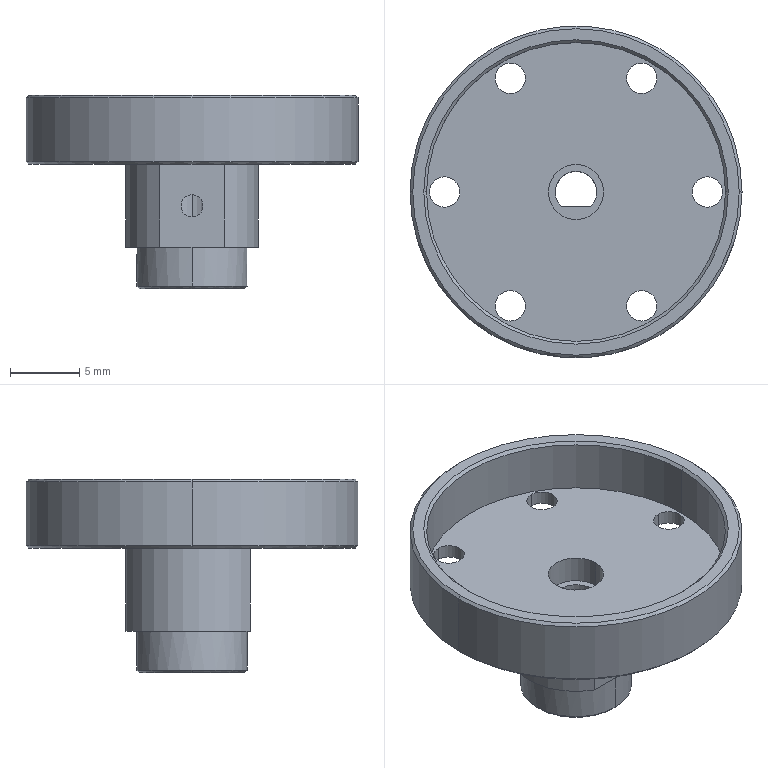Part | 1 solid | 49 faces | box 24 x 24 x 14 mm | volume 1249 mm3 | cylinder 29 | cone 12 | plane 8 | commonest cylinder face diameters 2.2 x12 1.25 x4 1.6 x2 3 x2 4 x2 8 x2
STEP:
#1=CARTESIAN_POINT('',(-11.8,0.,-5.));
#2=VERTEX_POINT('',#1);
#3=CARTESIAN_POINT('',(11.8,0.,-5.));
#4=VERTEX_POINT('',#3);
#5=CARTESIAN_POINT('',(0.,0.,-5.));
#6=DIRECTION('',(0.,0.,-1.));
#7=DIRECTION('',(0.,1.,0.));
#8=AXIS2_PLACEMENT_3D('',#5,#6,#7);
#9=CIRCLE('',#8,11.8);
#10=EDGE_CURVE('',#2,#4,#9,.T.);
#11=ORIENTED_EDGE('',*,*,#10,.F.);
#12=CARTESIAN_POINT('',(-12.,0.,-4.8));
#13=VERTEX_POINT('',#12);
#14=CARTESIAN_POINT('',(-12.,0.,-4.8));
#15=DIRECTION('',(-0.7071,0.,0.7071));
#16=VECTOR('',#15,1000.);
#17=LINE('',#14,#16);
#18=EDGE_CURVE('',#2,#13,#17,.T.);
#19=ORIENTED_EDGE('',*,*,#18,.T.);
#20=CARTESIAN_POINT('',(12.,0.,-4.8));
#21=VERTEX_POINT('',#20);
#22=CARTESIAN_POINT('',(0.,0.,-4.8));
#23=DIRECTION('',(0.,0.,1.));
#24=DIRECTION('',(-1.,0.,0.));
#25=AXIS2_PLACEMENT_3D('',#22,#23,#24);
#26=CIRCLE('',#25,12.);
#27=EDGE_CURVE('',#21,#13,#26,.T.);
#28=ORIENTED_EDGE('',*,*,#27,.F.);
#29=CARTESIAN_POINT('',(12.,0.,-4.8));
#30=DIRECTION('',(0.7071,0.,0.7071));
#31=VECTOR('',#30,1000.);
#32=LINE('',#29,#31);
#33=EDGE_CURVE('',#4,#21,#32,.T.);
#34=ORIENTED_EDGE('',*,*,#33,.F.);
#35=EDGE_LOOP('',(#11,#19,#28,#34));
#36=FACE_BOUND('',#35,.T.);
#37=CARTESIAN_POINT('',(0.,0.,-4.8));
#38=DIRECTION('',(0.,0.,1.));
#39=DIRECTION('',(-1.,0.,0.));
#40=AXIS2_PLACEMENT_3D('',#37,#38,#39);
#41=CONICAL_SURFACE('',#40,12.,0.7854);
#42=ADVANCED_FACE('',(#36),#41,.T.);
#43=CARTESIAN_POINT('',(-10.8,0.,-0.2));
#44=VERTEX_POINT('',#43);
#45=CARTESIAN_POINT('',(10.8,0.,-0.2));
#46=VERTEX_POINT('',#45);
#47=CARTESIAN_POINT('',(0.,0.,-0.2));
#48=DIRECTION('',(0.,0.,1.));
#49=DIRECTION('',(1.,0.,0.));
#50=AXIS2_PLACEMENT_3D('',#47,#48,#49);
#51=CIRCLE('',#50,10.8);
#52=EDGE_CURVE('',#44,#46,#51,.T.);
#53=ORIENTED_EDGE('',*,*,#52,.F.);
#54=CARTESIAN_POINT('',(-11.,0.,0.));
#55=VERTEX_POINT('',#54);
#56=CARTESIAN_POINT('',(-10.8,0.,-0.2));
#57=DIRECTION('',(-0.7071,0.,0.7071));
#58=VECTOR('',#57,1000.);
#59=LINE('',#56,#58);
#60=EDGE_CURVE('',#44,#55,#59,.T.);
#61=ORIENTED_EDGE('',*,*,#60,.T.);
#62=CARTESIAN_POINT('',(11.,0.,0.));
#63=VERTEX_POINT('',#62);
#64=CARTESIAN_POINT('',(0.,0.,0.));
#65=DIRECTION('',(0.,0.,-1.));
#66=DIRECTION('',(1.,0.,0.));
#67=AXIS2_PLACEMENT_3D('',#64,#65,#66);
#68=CIRCLE('',#67,11.);
#69=EDGE_CURVE('',#63,#55,#68,.T.);
#70=ORIENTED_EDGE('',*,*,#69,.F.);
#71=CARTESIAN_POINT('',(10.8,0.,-0.2));
#72=DIRECTION('',(0.7071,0.,0.7071));
#73=VECTOR('',#72,1000.);
#74=LINE('',#71,#73);
#75=EDGE_CURVE('',#46,#63,#74,.T.);
#76=ORIENTED_EDGE('',*,*,#75,.F.);
#77=EDGE_LOOP('',(#53,#61,#70,#76));
#78=FACE_BOUND('',#77,.T.);
#79=CARTESIAN_POINT('',(0.,0.,-0.2));
#80=DIRECTION('',(0.,0.,1.));
#81=DIRECTION('',(-1.,0.,0.));
#82=AXIS2_PLACEMENT_3D('',#79,#80,#81);
#83=CONICAL_SURFACE('',#82,10.8,0.7854);
#84=ADVANCED_FACE('',(#78),#83,.F.);
#85=CARTESIAN_POINT('',(11.8,0.,0.));
#86=VERTEX_POINT('',#85);
#87=CARTESIAN_POINT('',(-11.8,0.,0.));
#88=VERTEX_POINT('',#87);
#89=CARTESIAN_POINT('',(0.,0.,0.));
#90=DIRECTION('',(0.,0.,1.));
#91=DIRECTION('',(1.,0.,0.));
#92=AXIS2_PLACEMENT_3D('',#89,#90,#91);
#93=CIRCLE('',#92,11.8);
#94=EDGE_CURVE('',#86,#88,#93,.T.);
#95=ORIENTED_EDGE('',*,*,#94,.F.);
#96=CARTESIAN_POINT('',(12.,0.,-0.2));
#97=VERTEX_POINT('',#96);
#98=CARTESIAN_POINT('',(11.8,0.,0.));
#99=DIRECTION('',(0.7071,0.,-0.7071));
#100=VECTOR('',#99,1000.);
#101=LINE('',#98,#100);
#102=EDGE_CURVE('',#86,#97,#101,.T.);
#103=ORIENTED_EDGE('',*,*,#102,.T.);
#104=CARTESIAN_POINT('',(-12.,0.,-0.2));
#105=VERTEX_POINT('',#104);
#106=CARTESIAN_POINT('',(0.,0.,-0.2));
#107=DIRECTION('',(0.,0.,-1.));
#108=DIRECTION('',(1.,0.,0.));
#109=AXIS2_PLACEMENT_3D('',#106,#107,#108);
#110=CIRCLE('',#109,12.);
#111=EDGE_CURVE('',#105,#97,#110,.T.);
#112=ORIENTED_EDGE('',*,*,#111,.F.);
#113=CARTESIAN_POINT('',(-11.8,0.,0.));
#114=DIRECTION('',(-0.7071,0.,-0.7071));
#115=VECTOR('',#114,1000.);
#116=LINE('',#113,#115);
#117=EDGE_CURVE('',#88,#105,#116,.T.);
#118=ORIENTED_EDGE('',*,*,#117,.F.);
#119=EDGE_LOOP('',(#95,#103,#112,#118));
#120=FACE_BOUND('',#119,.T.);
#121=CARTESIAN_POINT('',(0.,0.,0.));
#122=DIRECTION('',(0.,0.,-1.));
#123=DIRECTION('',(1.,0.,0.));
#124=AXIS2_PLACEMENT_3D('',#121,#122,#123);
#125=CONICAL_SURFACE('',#124,11.8,0.7854);
#126=ADVANCED_FACE('',(#120),#125,.T.);
#127=CARTESIAN_POINT('',(-3.8,0.,-14.));
#128=VERTEX_POINT('',#127);
#129=CARTESIAN_POINT('',(3.8,0.,-14.));
#130=VERTEX_POINT('',#129);
#131=CARTESIAN_POINT('',(0.,0.,-14.));
#132=DIRECTION('',(0.,0.,-1.));
#133=DIRECTION('',(0.,1.,0.));
#134=AXIS2_PLACEMENT_3D('',#131,#132,#133);
#135=CIRCLE('',#134,3.8);
#136=EDGE_CURVE('',#128,#130,#135,.T.);
#137=ORIENTED_EDGE('',*,*,#136,.F.);
#138=CARTESIAN_POINT('',(-4.,0.,-13.8));
#139=VERTEX_POINT('',#138);
#140=CARTESIAN_POINT('',(-3.8,0.,-14.));
#141=DIRECTION('',(-0.7071,0.,0.7071));
#142=VECTOR('',#141,1000.);
#143=LINE('',#140,#142);
#144=EDGE_CURVE('',#128,#139,#143,.T.);
#145=ORIENTED_EDGE('',*,*,#144,.T.);
#146=CARTESIAN_POINT('',(0.,4.,-13.8));
#147=VERTEX_POINT('',#146);
#148=CARTESIAN_POINT('',(0.,0.,-13.8));
#149=DIRECTION('',(0.,0.,1.));
#150=DIRECTION('',(-1.,0.,0.));
#151=AXIS2_PLACEMENT_3D('',#148,#149,#150);
#152=CIRCLE('',#151,4.);
#153=EDGE_CURVE('',#147,#139,#152,.T.);
#154=ORIENTED_EDGE('',*,*,#153,.F.);
#155=CARTESIAN_POINT('',(4.,0.,-13.8));
#156=VERTEX_POINT('',#155);
#157=CARTESIAN_POINT('',(0.,0.,-13.8));
#158=DIRECTION('',(0.,0.,1.));
#159=DIRECTION('',(-1.,0.,0.));
#160=AXIS2_PLACEMENT_3D('',#157,#158,#159);
#161=CIRCLE('',#160,4.);
#162=EDGE_CURVE('',#156,#147,#161,.T.);
#163=ORIENTED_EDGE('',*,*,#162,.F.);
#164=CARTESIAN_POINT('',(3.8,0.,-14.));
#165=DIRECTION('',(0.7071,0.,0.7071));
#166=VECTOR('',#165,1000.);
#167=LINE('',#164,#166);
#168=EDGE_CURVE('',#130,#156,#167,.T.);
#169=ORIENTED_EDGE('',*,*,#168,.F.);
#170=EDGE_LOOP('',(#137,#145,#154,#163,#169));
#171=FACE_BOUND('',#170,.T.);
#172=CARTESIAN_POINT('',(0.,0.,-14.));
#173=DIRECTION('',(0.,0.,1.));
#174=DIRECTION('',(-1.,0.,0.));
#175=AXIS2_PLACEMENT_3D('',#172,#173,#174);
#176=CONICAL_SURFACE('',#175,3.8,0.7854);
#177=ADVANCED_FACE('',(#171),#176,.T.);
#178=CARTESIAN_POINT('',(-2.,0.,-6.));
#179=VERTEX_POINT('',#178);
#180=CARTESIAN_POINT('',(2.,0.,-6.));
#181=VERTEX_POINT('',#180);
#182=CARTESIAN_POINT('',(0.,0.,-6.));
#183=DIRECTION('',(0.,0.,1.));
#184=DIRECTION('',(1.,0.,0.));
#185=AXIS2_PLACEMENT_3D('',#182,#183,#184);
#186=CIRCLE('',#185,2.);
#187=EDGE_CURVE('',#179,#181,#186,.T.);
#188=ORIENTED_EDGE('',*,*,#187,.F.);
#189=CARTESIAN_POINT('',(-2.,0.,-4.));
#190=VERTEX_POINT('',#189);
#191=CARTESIAN_POINT('',(-2.,0.,-6.));
#192=DIRECTION('',(0.,0.,1.));
#193=VECTOR('',#192,1000.);
#194=LINE('',#191,#193);
#195=EDGE_CURVE('',#179,#190,#194,.T.);
#196=ORIENTED_EDGE('',*,*,#195,.T.);
#197=CARTESIAN_POINT('',(2.,0.,-4.));
#198=VERTEX_POINT('',#197);
#199=CARTESIAN_POINT('',(0.,0.,-4.));
#200=DIRECTION('',(0.,0.,1.));
#201=DIRECTION('',(1.,0.,0.));
#202=AXIS2_PLACEMENT_3D('',#199,#200,#201);
#203=CIRCLE('',#202,2.);
#204=EDGE_CURVE('',#190,#198,#203,.T.);
#205=ORIENTED_EDGE('',*,*,#204,.T.);
#206=CARTESIAN_POINT('',(2.,0.,-6.));
#207=DIRECTION('',(0.,0.,1.));
#208=VECTOR('',#207,1000.);
#209=LINE('',#206,#208);
#210=EDGE_CURVE('',#181,#198,#209,.T.);
#211=ORIENTED_EDGE('',*,*,#210,.F.);
#212=EDGE_LOOP('',(#188,#196,#205,#211));
#213=FACE_BOUND('',#212,.T.);
#214=CARTESIAN_POINT('',(0.,0.,-6.));
#215=DIRECTION('',(0.,0.,1.));
#216=DIRECTION('',(-1.,0.,0.));
#217=AXIS2_PLACEMENT_3D('',#214,#215,#216);
#218=CYLINDRICAL_SURFACE('',#217,2.);
#219=ADVANCED_FACE('',(#213),#218,.F.);
#220=ORIENTED_EDGE('',*,*,#111,.T.);
#221=CARTESIAN_POINT('',(12.,0.,0.));
#222=DIRECTION('',(0.,0.,-1.));
#223=VECTOR('',#222,1000.);
#224=LINE('',#221,#223);
#225=EDGE_CURVE('',#97,#21,#224,.T.);
#226=ORIENTED_EDGE('',*,*,#225,.T.);
#227=ORIENTED_EDGE('',*,*,#27,.T.);
#228=CARTESIAN_POINT('',(-12.,0.,0.));
#229=DIRECTION('',(0.,0.,-1.));
#230=VECTOR('',#229,1000.);
#231=LINE('',#228,#230);
#232=EDGE_CURVE('',#105,#13,#231,.T.);
#233=ORIENTED_EDGE('',*,*,#232,.F.);
#234=EDGE_LOOP('',(#220,#226,#227,#233));
#235=FACE_BOUND('',#234,.T.);
#236=CARTESIAN_POINT('',(0.,0.,0.));
#237=DIRECTION('',(0.,0.,-1.));
#238=DIRECTION('',(1.,0.,0.));
#239=AXIS2_PLACEMENT_3D('',#236,#237,#238);
#240=CYLINDRICAL_SURFACE('',#239,12.);
#241=ADVANCED_FACE('',(#235),#240,.T.);
#242=ORIENTED_EDGE('',*,*,#52,.T.);
#243=CARTESIAN_POINT('',(10.8,0.,-4.));
#244=VERTEX_POINT('',#243);
#245=CARTESIAN_POINT('',(10.8,0.,0.));
#246=DIRECTION('',(0.,0.,-1.));
#247=VECTOR('',#246,1000.);
#248=LINE('',#245,#247);
#249=EDGE_CURVE('',#46,#244,#248,.T.);
#250=ORIENTED_EDGE('',*,*,#249,.T.);
#251=CARTESIAN_POINT('',(-10.8,0.,-4.));
#252=VERTEX_POINT('',#251);
#253=CARTESIAN_POINT('',(0.,0.,-4.));
#254=DIRECTION('',(0.,0.,-1.));
#255=DIRECTION('',(0.,1.,0.));
#256=AXIS2_PLACEMENT_3D('',#253,#254,#255);
#257=CIRCLE('',#256,10.8);
#258=EDGE_CURVE('',#244,#252,#257,.T.);
#259=ORIENTED_EDGE('',*,*,#258,.T.);
#260=CARTESIAN_POINT('',(-10.8,0.,0.));
#261=DIRECTION('',(0.,0.,-1.));
#262=VECTOR('',#261,1000.);
#263=LINE('',#260,#262);
#264=EDGE_CURVE('',#44,#252,#263,.T.);
#265=ORIENTED_EDGE('',*,*,#264,.F.);
#266=EDGE_LOOP('',(#242,#250,#259,#265));
#267=FACE_BOUND('',#266,.T.);
#268=CARTESIAN_POINT('',(0.,0.,0.));
#269=DIRECTION('',(0.,0.,-1.));
#270=DIRECTION('',(1.,0.,0.));
#271=AXIS2_PLACEMENT_3D('',#268,#269,#270);
#272=CYLINDRICAL_SURFACE('',#271,10.8);
#273=ADVANCED_FACE('',(#267),#272,.F.);
#274=CARTESIAN_POINT('',(-2.75,-0.625,-9.75));
#275=VERTEX_POINT('',#274);
#276=CARTESIAN_POINT('',(-2.75,0.625,-9.75));
#277=VERTEX_POINT('',#276);
#278=CARTESIAN_POINT('',(-2.75,0.,-9.75));
#279=DIRECTION('',(0.,0.,-1.));
#280=DIRECTION('',(0.,1.,0.));
#281=AXIS2_PLACEMENT_3D('',#278,#279,#280);
#282=CIRCLE('',#281,0.625);
#283=EDGE_CURVE('',#275,#277,#282,.T.);
#284=ORIENTED_EDGE('',*,*,#283,.F.);
#285=CARTESIAN_POINT('',(-2.75,-0.625,-14.));
#286=VERTEX_POINT('',#285);
#287=CARTESIAN_POINT('',(-2.75,-0.625,-14.));
#288=DIRECTION('',(0.,0.,-1.));
#289=VECTOR('',#288,1000.);
#290=LINE('',#287,#289);
#291=EDGE_CURVE('',#275,#286,#290,.T.);
#292=ORIENTED_EDGE('',*,*,#291,.T.);
#293=CARTESIAN_POINT('',(-2.75,0.625,-14.));
#294=VERTEX_POINT('',#293);
#295=CARTESIAN_POINT('',(-2.75,0.,-14.));
#296=DIRECTION('',(0.,0.,-1.));
#297=DIRECTION('',(0.,1.,0.));
#298=AXIS2_PLACEMENT_3D('',#295,#296,#297);
#299=CIRCLE('',#298,0.625);
#300=EDGE_CURVE('',#286,#294,#299,.T.);
#301=ORIENTED_EDGE('',*,*,#300,.T.);
#302=CARTESIAN_POINT('',(-2.75,0.625,-14.));
#303=DIRECTION('',(0.,0.,-1.));
#304=VECTOR('',#303,1000.);
#305=LINE('',#302,#304);
#306=EDGE_CURVE('',#277,#294,#305,.T.);
#307=ORIENTED_EDGE('',*,*,#306,.F.);
#308=EDGE_LOOP('',(#284,#292,#301,#307));
#309=FACE_BOUND('',#308,.T.);
#310=CARTESIAN_POINT('',(-2.75,0.,-14.));
#311=DIRECTION('',(0.,0.,-1.));
#312=DIRECTION('',(0.,-1.,0.));
#313=AXIS2_PLACEMENT_3D('',#310,#311,#312);
#314=CYLINDRICAL_SURFACE('',#313,0.625);
#315=ADVANCED_FACE('',(#309),#314,.F.);
#316=CARTESIAN_POINT('',(-2.75,0.,-9.374));
#317=VERTEX_POINT('',#316);
#318=CARTESIAN_POINT('',(-2.75,0.625,-9.75));
#319=DIRECTION('',(0.,0.8572,-0.515));
#320=VECTOR('',#319,1000.);
#321=LINE('',#318,#320);
#322=EDGE_CURVE('',#317,#277,#321,.T.);
#323=ORIENTED_EDGE('',*,*,#322,.F.);
#324=CARTESIAN_POINT('',(-2.75,-0.625,-9.75));
#325=DIRECTION('',(0.,-0.8572,-0.515));
#326=VECTOR('',#325,1000.);
#327=LINE('',#324,#326);
#328=EDGE_CURVE('',#317,#275,#327,.T.);
#329=ORIENTED_EDGE('',*,*,#328,.T.);
#330=ORIENTED_EDGE('',*,*,#283,.T.);
#331=EDGE_LOOP('',(#323,#329,#330));
#332=FACE_BOUND('',#331,.T.);
#333=CARTESIAN_POINT('',(-2.75,0.,-9.75));
#334=DIRECTION('',(0.,0.,-1.));
#335=DIRECTION('',(0.,-1.,0.));
#336=AXIS2_PLACEMENT_3D('',#333,#334,#335);
#337=CONICAL_SURFACE('',#336,0.625,1.03);
#338=ADVANCED_FACE('',(#332),#337,.F.);
#339=CARTESIAN_POINT('',(2.75,-0.625,-9.75));
#340=VERTEX_POINT('',#339);
#341=CARTESIAN_POINT('',(2.75,0.625,-9.75));
#342=VERTEX_POINT('',#341);
#343=CARTESIAN_POINT('',(2.75,0.,-9.75));
#344=DIRECTION('',(0.,0.,-1.));
#345=DIRECTION('',(0.,1.,0.));
#346=AXIS2_PLACEMENT_3D('',#343,#344,#345);
#347=CIRCLE('',#346,0.625);
#348=EDGE_CURVE('',#340,#342,#347,.T.);
#349=ORIENTED_EDGE('',*,*,#348,.F.);
#350=CARTESIAN_POINT('',(2.75,-0.625,-14.));
#351=VERTEX_POINT('',#350);
#352=CARTESIAN_POINT('',(2.75,-0.625,-14.));
#353=DIRECTION('',(0.,0.,-1.));
#354=VECTOR('',#353,1000.);
#355=LINE('',#352,#354);
#356=EDGE_CURVE('',#340,#351,#355,.T.);
#357=ORIENTED_EDGE('',*,*,#356,.T.);
#358=CARTESIAN_POINT('',(2.75,0.625,-14.));
#359=VERTEX_POINT('',#358);
#360=CARTESIAN_POINT('',(2.75,0.,-14.));
#361=DIRECTION('',(0.,0.,-1.));
#362=DIRECTION('',(0.,1.,0.));
#363=AXIS2_PLACEMENT_3D('',#360,#361,#362);
#364=CIRCLE('',#363,0.625);
#365=EDGE_CURVE('',#351,#359,#364,.T.);
#366=ORIENTED_EDGE('',*,*,#365,.T.);
#367=CARTESIAN_POINT('',(2.75,0.625,-14.));
#368=DIRECTION('',(0.,0.,-1.));
#369=VECTOR('',#368,1000.);
#370=LINE('',#367,#369);
#371=EDGE_CURVE('',#342,#359,#370,.T.);
#372=ORIENTED_EDGE('',*,*,#371,.F.);
#373=EDGE_LOOP('',(#349,#357,#366,#372));
#374=FACE_BOUND('',#373,.T.);
#375=CARTESIAN_POINT('',(2.75,0.,-14.));
#376=DIRECTION('',(0.,0.,-1.));
#377=DIRECTION('',(0.,-1.,0.));
#378=AXIS2_PLACEMENT_3D('',#375,#376,#377);
#379=CYLINDRICAL_SURFACE('',#378,0.625);
#380=ADVANCED_FACE('',(#374),#379,.F.);
#381=CARTESIAN_POINT('',(2.75,0.,-9.374));
#382=VERTEX_POINT('',#381);
#383=CARTESIAN_POINT('',(2.75,0.625,-9.75));
#384=DIRECTION('',(0.,0.8572,-0.515));
#385=VECTOR('',#384,1000.);
#386=LINE('',#383,#385);
#387=EDGE_CURVE('',#382,#342,#386,.T.);
#388=ORIENTED_EDGE('',*,*,#387,.F.);
#389=CARTESIAN_POINT('',(2.75,-0.625,-9.75));
#390=DIRECTION('',(0.,-0.8572,-0.515));
#391=VECTOR('',#390,1000.);
#392=LINE('',#389,#391);
#393=EDGE_CURVE('',#382,#340,#392,.T.);
#394=ORIENTED_EDGE('',*,*,#393,.T.);
#395=ORIENTED_EDGE('',*,*,#348,.T.);
#396=EDGE_LOOP('',(#388,#394,#395));
#397=FACE_BOUND('',#396,.T.);
#398=CARTESIAN_POINT('',(2.75,0.,-9.75));
#399=DIRECTION('',(0.,0.,-1.));
#400=DIRECTION('',(0.,-1.,0.));
#401=AXIS2_PLACEMENT_3D('',#398,#399,#400);
#402=CONICAL_SURFACE('',#401,0.625,1.03);
#403=ADVANCED_FACE('',(#397),#402,.F.);
#404=CARTESIAN_POINT('',(0.,-1.05,-7.2));
#405=VERTEX_POINT('',#404);
#406=CARTESIAN_POINT('',(0.,-1.05,-8.8));
#407=VERTEX_POINT('',#406);
#408=CARTESIAN_POINT('',(0.,-1.05,-8.));
#409=DIRECTION('',(0.,-1.,0.));
#410=DIRECTION('',(0.,0.,-1.));
#411=AXIS2_PLACEMENT_3D('',#408,#409,#410);
#412=CIRCLE('',#411,0.8);
#413=EDGE_CURVE('',#405,#407,#412,.T.);
#414=ORIENTED_EDGE('',*,*,#413,.F.);
#415=CARTESIAN_POINT('',(0.,-4.2,-7.2));
#416=VERTEX_POINT('',#415);
#417=CARTESIAN_POINT('',(0.,-4.2,-7.2));
#418=DIRECTION('',(0.,-1.,0.));
#419=VECTOR('',#418,1000.);
#420=LINE('',#417,#419);
#421=EDGE_CURVE('',#405,#416,#420,.T.);
#422=ORIENTED_EDGE('',*,*,#421,.T.);
#423=CARTESIAN_POINT('',(0.,-4.2,-8.8));
#424=VERTEX_POINT('',#423);
#425=CARTESIAN_POINT('',(0.,-4.2,-8.));
#426=DIRECTION('',(0.,-1.,0.));
#427=DIRECTION('',(0.,0.,-1.));
#428=AXIS2_PLACEMENT_3D('',#425,#426,#427);
#429=CIRCLE('',#428,0.8);
#430=EDGE_CURVE('',#416,#424,#429,.T.);
#431=ORIENTED_EDGE('',*,*,#430,.T.);
#432=CARTESIAN_POINT('',(0.,-4.2,-8.8));
#433=DIRECTION('',(0.,-1.,0.));
#434=VECTOR('',#433,1000.);
#435=LINE('',#432,#434);
#436=EDGE_CURVE('',#407,#424,#435,.T.);
#437=ORIENTED_EDGE('',*,*,#436,.F.);
#438=EDGE_LOOP('',(#414,#422,#431,#437));
#439=FACE_BOUND('',#438,.T.);
#440=CARTESIAN_POINT('',(0.,-4.2,-8.));
#441=DIRECTION('',(0.,-1.,0.));
#442=DIRECTION('',(0.,0.,1.));
#443=AXIS2_PLACEMENT_3D('',#440,#441,#442);
#444=CYLINDRICAL_SURFACE('',#443,0.8);
#445=ADVANCED_FACE('',(#439),#444,.F.);
#446=CARTESIAN_POINT('',(0.,-4.,-13.8));
#447=VERTEX_POINT('',#446);
#448=CARTESIAN_POINT('',(0.,0.,-13.8));
#449=DIRECTION('',(0.,0.,1.));
#450=DIRECTION('',(-1.,0.,0.));
#451=AXIS2_PLACEMENT_3D('',#448,#449,#450);
#452=CIRCLE('',#451,4.);
#453=EDGE_CURVE('',#447,#156,#452,.T.);
#454=ORIENTED_EDGE('',*,*,#453,.T.);
#455=ORIENTED_EDGE('',*,*,#162,.T.);
#456=CARTESIAN_POINT('',(0.,4.,-11.));
#457=VERTEX_POINT('',#456);
#458=CARTESIAN_POINT('',(0.,4.,-14.));
#459=DIRECTION('',(0.,0.,1.));
#460=VECTOR('',#459,1000.);
#461=LINE('',#458,#460);
#462=EDGE_CURVE('',#147,#457,#461,.T.);
#463=ORIENTED_EDGE('',*,*,#462,.T.);
#464=CARTESIAN_POINT('',(0.,-4.,-11.));
#465=VERTEX_POINT('',#464);
#466=CARTESIAN_POINT('',(0.,0.,-11.));
#467=DIRECTION('',(0.,0.,-1.));
#468=DIRECTION('',(0.,1.,0.));
#469=AXIS2_PLACEMENT_3D('',#466,#467,#468);
#470=CIRCLE('',#469,4.);
#471=EDGE_CURVE('',#457,#465,#470,.T.);
#472=ORIENTED_EDGE('',*,*,#471,.T.);
#473=CARTESIAN_POINT('',(0.,-4.,-14.));
#474=DIRECTION('',(0.,0.,1.));
#475=VECTOR('',#474,1000.);
#476=LINE('',#473,#475);
#477=EDGE_CURVE('',#447,#465,#476,.T.);
#478=ORIENTED_EDGE('',*,*,#477,.F.);
#479=EDGE_LOOP('',(#454,#455,#463,#472,#478));
#480=FACE_BOUND('',#479,.T.);
#481=CARTESIAN_POINT('',(0.,0.,-14.));
#482=DIRECTION('',(0.,0.,1.));
#483=DIRECTION('',(0.,1.,0.));
#484=AXIS2_PLACEMENT_3D('',#481,#482,#483);
#485=CYLINDRICAL_SURFACE('',#484,4.);
#486=ADVANCED_FACE('',(#480),#485,.T.);
#487=CARTESIAN_POINT('',(-4.75,7.127,-5.));
#488=VERTEX_POINT('',#487);
#489=CARTESIAN_POINT('',(-4.75,9.327,-5.));
#490=VERTEX_POINT('',#489);
#491=CARTESIAN_POINT('',(-4.75,8.227,-5.));
#492=DIRECTION('',(0.,0.,-1.));
#493=DIRECTION('',(0.,1.,0.));
#494=AXIS2_PLACEMENT_3D('',#491,#492,#493);
#495=CIRCLE('',#494,1.1);
#496=EDGE_CURVE('',#488,#490,#495,.T.);
#497=ORIENTED_EDGE('',*,*,#496,.T.);
#498=CARTESIAN_POINT('',(-4.75,9.327,-4.));
#499=VERTEX_POINT('',#498);
#500=CARTESIAN_POINT('',(-4.75,9.327,-5.));
#501=DIRECTION('',(0.,0.,1.));
#502=VECTOR('',#501,1000.);
#503=LINE('',#500,#502);
#504=EDGE_CURVE('',#490,#499,#503,.T.);
#505=ORIENTED_EDGE('',*,*,#504,.T.);
#506=CARTESIAN_POINT('',(-4.75,7.127,-4.));
#507=VERTEX_POINT('',#506);
#508=CARTESIAN_POINT('',(-4.75,8.227,-4.));
#509=DIRECTION('',(0.,0.,-1.));
#510=DIRECTION('',(0.,1.,0.));
#511=AXIS2_PLACEMENT_3D('',#508,#509,#510);
#512=CIRCLE('',#511,1.1);
#513=EDGE_CURVE('',#507,#499,#512,.T.);
#514=ORIENTED_EDGE('',*,*,#513,.F.);
#515=CARTESIAN_POINT('',(-4.75,7.127,-5.));
#516=DIRECTION('',(0.,0.,1.));
#517=VECTOR('',#516,1000.);
#518=LINE('',#515,#517);
#519=EDGE_CURVE('',#488,#507,#518,.T.);
#520=ORIENTED_EDGE('',*,*,#519,.F.);
#521=EDGE_LOOP('',(#497,#505,#514,#520));
#522=FACE_BOUND('',#521,.T.);
#523=CARTESIAN_POINT('',(-4.75,8.227,-5.));
#524=DIRECTION('',(0.,0.,1.));
#525=DIRECTION('',(0.,1.,0.));
#526=AXIS2_PLACEMENT_3D('',#523,#524,#525);
#527=CYLINDRICAL_SURFACE('',#526,1.1);
#528=ADVANCED_FACE('',(#522),#527,.F.);
#529=CARTESIAN_POINT('',(4.75,7.127,-5.));
#530=VERTEX_POINT('',#529);
#531=CARTESIAN_POINT('',(4.75,9.327,-5.));
#532=VERTEX_POINT('',#531);
#533=CARTESIAN_POINT('',(4.75,8.227,-5.));
#534=DIRECTION('',(0.,0.,-1.));
#535=DIRECTION('',(0.,1.,0.));
#536=AXIS2_PLACEMENT_3D('',#533,#534,#535);
#537=CIRCLE('',#536,1.1);
#538=EDGE_CURVE('',#530,#532,#537,.T.);
#539=ORIENTED_EDGE('',*,*,#538,.T.);
#540=CARTESIAN_POINT('',(4.75,9.327,-4.));
#541=VERTEX_POINT('',#540);
#542=CARTESIAN_POINT('',(4.75,9.327,-5.));
#543=DIRECTION('',(0.,0.,1.));
#544=VECTOR('',#543,1000.);
#545=LINE('',#542,#544);
#546=EDGE_CURVE('',#532,#541,#545,.T.);
#547=ORIENTED_EDGE('',*,*,#546,.T.);
#548=CARTESIAN_POINT('',(4.75,7.127,-4.));
#549=VERTEX_POINT('',#548);
#550=CARTESIAN_POINT('',(4.75,8.227,-4.));
#551=DIRECTION('',(0.,0.,-1.));
#552=DIRECTION('',(0.,1.,0.));
#553=AXIS2_PLACEMENT_3D('',#550,#551,#552);
#554=CIRCLE('',#553,1.1);
#555=EDGE_CURVE('',#549,#541,#554,.T.);
#556=ORIENTED_EDGE('',*,*,#555,.F.);
#557=CARTESIAN_POINT('',(4.75,7.127,-5.));
#558=DIRECTION('',(0.,0.,1.));
#559=VECTOR('',#558,1000.);
#560=LINE('',#557,#559);
#561=EDGE_CURVE('',#530,#549,#560,.T.);
#562=ORIENTED_EDGE('',*,*,#561,.F.);
#563=EDGE_LOOP('',(#539,#547,#556,#562));
#564=FACE_BOUND('',#563,.T.);
#565=CARTESIAN_POINT('',(4.75,8.227,-5.));
#566=DIRECTION('',(0.,0.,1.));
#567=DIRECTION('',(0.,1.,0.));
#568=AXIS2_PLACEMENT_3D('',#565,#566,#567);
#569=CYLINDRICAL_SURFACE('',#568,1.1);
#570=ADVANCED_FACE('',(#564),#569,.F.);
#571=CARTESIAN_POINT('',(9.5,-1.1,-5.));
#572=VERTEX_POINT('',#571);
#573=CARTESIAN_POINT('',(9.5,1.1,-5.));
#574=VERTEX_POINT('',#573);
#575=CARTESIAN_POINT('',(9.5,0.,-5.));
#576=DIRECTION('',(0.,0.,-1.));
#577=DIRECTION('',(0.,1.,0.));
#578=AXIS2_PLACEMENT_3D('',#575,#576,#577);
#579=CIRCLE('',#578,1.1);
#580=EDGE_CURVE('',#572,#574,#579,.T.);
#581=ORIENTED_EDGE('',*,*,#580,.T.);
#582=CARTESIAN_POINT('',(9.5,1.1,-4.));
#583=VERTEX_POINT('',#582);
#584=CARTESIAN_POINT('',(9.5,1.1,-5.));
#585=DIRECTION('',(0.,0.,1.));
#586=VECTOR('',#585,1000.);
#587=LINE('',#584,#586);
#588=EDGE_CURVE('',#574,#583,#587,.T.);
#589=ORIENTED_EDGE('',*,*,#588,.T.);
#590=CARTESIAN_POINT('',(9.5,-1.1,-4.));
#591=VERTEX_POINT('',#590);
#592=CARTESIAN_POINT('',(9.5,0.,-4.));
#593=DIRECTION('',(0.,0.,-1.));
#594=DIRECTION('',(0.,1.,0.));
#595=AXIS2_PLACEMENT_3D('',#592,#593,#594);
#596=CIRCLE('',#595,1.1);
#597=EDGE_CURVE('',#591,#583,#596,.T.);
#598=ORIENTED_EDGE('',*,*,#597,.F.);
#599=CARTESIAN_POINT('',(9.5,-1.1,-5.));
#600=DIRECTION('',(0.,0.,1.));
#601=VECTOR('',#600,1000.);
#602=LINE('',#599,#601);
#603=EDGE_CURVE('',#572,#591,#602,.T.);
#604=ORIENTED_EDGE('',*,*,#603,.F.);
#605=EDGE_LOOP('',(#581,#589,#598,#604));
#606=FACE_BOUND('',#605,.T.);
#607=CARTESIAN_POINT('',(9.5,0.,-5.));
#608=DIRECTION('',(0.,0.,1.));
#609=DIRECTION('',(0.,1.,0.));
#610=AXIS2_PLACEMENT_3D('',#607,#608,#609);
#611=CYLINDRICAL_SURFACE('',#610,1.1);
#612=ADVANCED_FACE('',(#606),#611,.F.);
#613=CARTESIAN_POINT('',(4.75,-9.327,-5.));
#614=VERTEX_POINT('',#613);
#615=CARTESIAN_POINT('',(4.75,-7.127,-5.));
#616=VERTEX_POINT('',#615);
#617=CARTESIAN_POINT('',(4.75,-8.227,-5.));
#618=DIRECTION('',(0.,0.,-1.));
#619=DIRECTION('',(0.,1.,0.));
#620=AXIS2_PLACEMENT_3D('',#617,#618,#619);
#621=CIRCLE('',#620,1.1);
#622=EDGE_CURVE('',#614,#616,#621,.T.);
#623=ORIENTED_EDGE('',*,*,#622,.T.);
#624=CARTESIAN_POINT('',(4.75,-7.127,-4.));
#625=VERTEX_POINT('',#624);
#626=CARTESIAN_POINT('',(4.75,-7.127,-5.));
#627=DIRECTION('',(0.,0.,1.));
#628=VECTOR('',#627,1000.);
#629=LINE('',#626,#628);
#630=EDGE_CURVE('',#616,#625,#629,.T.);
#631=ORIENTED_EDGE('',*,*,#630,.T.);
#632=CARTESIAN_POINT('',(4.75,-9.327,-4.));
#633=VERTEX_POINT('',#632);
#634=CARTESIAN_POINT('',(4.75,-8.227,-4.));
#635=DIRECTION('',(0.,0.,-1.));
#636=DIRECTION('',(0.,1.,0.));
#637=AXIS2_PLACEMENT_3D('',#634,#635,#636);
#638=CIRCLE('',#637,1.1);
#639=EDGE_CURVE('',#633,#625,#638,.T.);
#640=ORIENTED_EDGE('',*,*,#639,.F.);
#641=CARTESIAN_POINT('',(4.75,-9.327,-5.));
#642=DIRECTION('',(0.,0.,1.));
#643=VECTOR('',#642,1000.);
#644=LINE('',#641,#643);
#645=EDGE_CURVE('',#614,#633,#644,.T.);
#646=ORIENTED_EDGE('',*,*,#645,.F.);
#647=EDGE_LOOP('',(#623,#631,#640,#646));
#648=FACE_BOUND('',#647,.T.);
#649=CARTESIAN_POINT('',(4.75,-8.227,-5.));
#650=DIRECTION('',(0.,0.,1.));
#651=DIRECTION('',(0.,1.,0.));
#652=AXIS2_PLACEMENT_3D('',#649,#650,#651);
#653=CYLINDRICAL_SURFACE('',#652,1.1);
#654=ADVANCED_FACE('',(#648),#653,.F.);
#655=CARTESIAN_POINT('',(-4.75,-9.327,-5.));
#656=VERTEX_POINT('',#655);
#657=CARTESIAN_POINT('',(-4.75,-7.127,-5.));
#658=VERTEX_POINT('',#657);
#659=CARTESIAN_POINT('',(-4.75,-8.227,-5.));
#660=DIRECTION('',(0.,0.,-1.));
#661=DIRECTION('',(0.,1.,0.));
#662=AXIS2_PLACEMENT_3D('',#659,#660,#661);
#663=CIRCLE('',#662,1.1);
#664=EDGE_CURVE('',#656,#658,#663,.T.);
#665=ORIENTED_EDGE('',*,*,#664,.T.);
#666=CARTESIAN_POINT('',(-4.75,-7.127,-4.));
#667=VERTEX_POINT('',#666);
#668=CARTESIAN_POINT('',(-4.75,-7.127,-5.));
#669=DIRECTION('',(0.,0.,1.));
#670=VECTOR('',#669,1000.);
#671=LINE('',#668,#670);
#672=EDGE_CURVE('',#658,#667,#671,.T.);
#673=ORIENTED_EDGE('',*,*,#672,.T.);
#674=CARTESIAN_POINT('',(-4.75,-9.327,-4.));
#675=VERTEX_POINT('',#674);
#676=CARTESIAN_POINT('',(-4.75,-8.227,-4.));
#677=DIRECTION('',(0.,0.,-1.));
#678=DIRECTION('',(0.,1.,0.));
#679=AXIS2_PLACEMENT_3D('',#676,#677,#678);
#680=CIRCLE('',#679,1.1);
#681=EDGE_CURVE('',#675,#667,#680,.T.);
#682=ORIENTED_EDGE('',*,*,#681,.F.);
#683=CARTESIAN_POINT('',(-4.75,-9.327,-5.));
#684=DIRECTION('',(0.,0.,1.));
#685=VECTOR('',#684,1000.);
#686=LINE('',#683,#685);
#687=EDGE_CURVE('',#656,#675,#686,.T.);
#688=ORIENTED_EDGE('',*,*,#687,.F.);
#689=EDGE_LOOP('',(#665,#673,#682,#688));
#690=FACE_BOUND('',#689,.T.);
#691=CARTESIAN_POINT('',(-4.75,-8.227,-5.));
#692=DIRECTION('',(0.,0.,1.));
#693=DIRECTION('',(0.,1.,0.));
#694=AXIS2_PLACEMENT_3D('',#691,#692,#693);
#695=CYLINDRICAL_SURFACE('',#694,1.1);
#696=ADVANCED_FACE('',(#690),#695,.F.);
#697=CARTESIAN_POINT('',(-9.5,-1.1,-5.));
#698=VERTEX_POINT('',#697);
#699=CARTESIAN_POINT('',(-9.5,1.1,-5.));
#700=VERTEX_POINT('',#699);
#701=CARTESIAN_POINT('',(-9.5,0.,-5.));
#702=DIRECTION('',(0.,0.,-1.));
#703=DIRECTION('',(0.,1.,0.));
#704=AXIS2_PLACEMENT_3D('',#701,#702,#703);
#705=CIRCLE('',#704,1.1);
#706=EDGE_CURVE('',#698,#700,#705,.T.);
#707=ORIENTED_EDGE('',*,*,#706,.T.);
#708=CARTESIAN_POINT('',(-9.5,1.1,-4.));
#709=VERTEX_POINT('',#708);
#710=CARTESIAN_POINT('',(-9.5,1.1,-5.));
#711=DIRECTION('',(0.,0.,1.));
#712=VECTOR('',#711,1000.);
#713=LINE('',#710,#712);
#714=EDGE_CURVE('',#700,#709,#713,.T.);
#715=ORIENTED_EDGE('',*,*,#714,.T.);
#716=CARTESIAN_POINT('',(-9.5,-1.1,-4.));
#717=VERTEX_POINT('',#716);
#718=CARTESIAN_POINT('',(-9.5,0.,-4.));
#719=DIRECTION('',(0.,0.,-1.));
#720=DIRECTION('',(0.,1.,0.));
#721=AXIS2_PLACEMENT_3D('',#718,#719,#720);
#722=CIRCLE('',#721,1.1);
#723=EDGE_CURVE('',#717,#709,#722,.T.);
#724=ORIENTED_EDGE('',*,*,#723,.F.);
#725=CARTESIAN_POINT('',(-9.5,-1.1,-5.));
#726=DIRECTION('',(0.,0.,1.));
#727=VECTOR('',#726,1000.);
#728=LINE('',#725,#727);
#729=EDGE_CURVE('',#698,#717,#728,.T.);
#730=ORIENTED_EDGE('',*,*,#729,.F.);
#731=EDGE_LOOP('',(#707,#715,#724,#730));
#732=FACE_BOUND('',#731,.T.);
#733=CARTESIAN_POINT('',(-9.5,0.,-5.));
#734=DIRECTION('',(0.,0.,1.));
#735=DIRECTION('',(0.,1.,0.));
#736=AXIS2_PLACEMENT_3D('',#733,#734,#735);
#737=CYLINDRICAL_SURFACE('',#736,1.1);
#738=ADVANCED_FACE('',(#732),#737,.F.);
#739=CARTESIAN_POINT('',(0.,1.5,-6.));
#740=VERTEX_POINT('',#739);
#741=CARTESIAN_POINT('',(1.071,-1.05,-6.));
#742=VERTEX_POINT('',#741);
#743=CARTESIAN_POINT('',(0.,0.,-6.));
#744=DIRECTION('',(0.,0.,-1.));
#745=DIRECTION('',(1.,0.,0.));
#746=AXIS2_PLACEMENT_3D('',#743,#744,#745);
#747=CIRCLE('',#746,1.5);
#748=EDGE_CURVE('',#740,#742,#747,.T.);
#749=ORIENTED_EDGE('',*,*,#748,.F.);
#750=CARTESIAN_POINT('',(0.,1.5,-14.));
#751=VERTEX_POINT('',#750);
#752=CARTESIAN_POINT('',(0.,1.5,56.5));
#753=DIRECTION('',(0.,0.,-1.));
#754=VECTOR('',#753,1000.);
#755=LINE('',#752,#754);
#756=EDGE_CURVE('',#740,#751,#755,.T.);
#757=ORIENTED_EDGE('',*,*,#756,.T.);
#758=CARTESIAN_POINT('',(1.071,-1.05,-14.));
#759=VERTEX_POINT('',#758);
#760=CARTESIAN_POINT('',(0.,0.,-14.));
#761=DIRECTION('',(0.,0.,-1.));
#762=DIRECTION('',(0.,1.,0.));
#763=AXIS2_PLACEMENT_3D('',#760,#761,#762);
#764=CIRCLE('',#763,1.5);
#765=EDGE_CURVE('',#751,#759,#764,.T.);
#766=ORIENTED_EDGE('',*,*,#765,.T.);
#767=CARTESIAN_POINT('',(1.071,-1.05,56.5));
#768=DIRECTION('',(0.,0.,-1.));
#769=VECTOR('',#768,1000.);
#770=LINE('',#767,#769);
#771=EDGE_CURVE('',#742,#759,#770,.T.);
#772=ORIENTED_EDGE('',*,*,#771,.F.);
#773=EDGE_LOOP('',(#749,#757,#766,#772));
#774=FACE_BOUND('',#773,.T.);
#775=CARTESIAN_POINT('',(0.,0.,56.5));
#776=DIRECTION('',(0.,0.,-1.));
#777=DIRECTION('',(0.,-1.,0.));
#778=AXIS2_PLACEMENT_3D('',#775,#776,#777);
#779=CYLINDRICAL_SURFACE('',#778,1.5);
#780=ADVANCED_FACE('',(#774),#779,.F.);
#781=ORIENTED_EDGE('',*,*,#756,.F.);
#782=CARTESIAN_POINT('',(-1.071,-1.05,-6.));
#783=VERTEX_POINT('',#782);
#784=CARTESIAN_POINT('',(0.,0.,-6.));
#785=DIRECTION('',(0.,0.,-1.));
#786=DIRECTION('',(1.,0.,0.));
#787=AXIS2_PLACEMENT_3D('',#784,#785,#786);
#788=CIRCLE('',#787,1.5);
#789=EDGE_CURVE('',#783,#740,#788,.T.);
#790=ORIENTED_EDGE('',*,*,#789,.F.);
#791=CARTESIAN_POINT('',(-1.071,-1.05,-14.));
#792=VERTEX_POINT('',#791);
#793=CARTESIAN_POINT('',(-1.071,-1.05,56.5));
#794=DIRECTION('',(0.,0.,-1.));
#795=VECTOR('',#794,1000.);
#796=LINE('',#793,#795);
#797=EDGE_CURVE('',#783,#792,#796,.T.);
#798=ORIENTED_EDGE('',*,*,#797,.T.);
#799=CARTESIAN_POINT('',(0.,0.,-14.));
#800=DIRECTION('',(0.,0.,-1.));
#801=DIRECTION('',(0.,1.,0.));
#802=AXIS2_PLACEMENT_3D('',#799,#800,#801);
#803=CIRCLE('',#802,1.5);
#804=EDGE_CURVE('',#792,#751,#803,.T.);
#805=ORIENTED_EDGE('',*,*,#804,.T.);
#806=EDGE_LOOP('',(#781,#790,#798,#805));
#807=FACE_BOUND('',#806,.T.);
#808=CARTESIAN_POINT('',(0.,0.,56.5));
#809=DIRECTION('',(0.,0.,-1.));
#810=DIRECTION('',(0.,-1.,0.));
#811=AXIS2_PLACEMENT_3D('',#808,#809,#810);
#812=CYLINDRICAL_SURFACE('',#811,1.5);
#813=ADVANCED_FACE('',(#807),#812,.F.);
#814=CARTESIAN_POINT('',(0.,-1.05,-8.));
#815=DIRECTION('',(0.,-1.,0.));
#816=DIRECTION('',(0.,0.,-1.));
#817=AXIS2_PLACEMENT_3D('',#814,#815,#816);
#818=CIRCLE('',#817,0.8);
#819=EDGE_CURVE('',#407,#405,#818,.T.);
#820=ORIENTED_EDGE('',*,*,#819,.T.);
#821=ORIENTED_EDGE('',*,*,#413,.T.);
#822=EDGE_LOOP('',(#820,#821));
#823=FACE_BOUND('',#822,.T.);
#824=CARTESIAN_POINT('',(1.071,-1.05,-6.));
#825=DIRECTION('',(-1.,0.,0.));
#826=VECTOR('',#825,1000.);
#827=LINE('',#824,#826);
#828=EDGE_CURVE('',#742,#783,#827,.T.);
#829=ORIENTED_EDGE('',*,*,#828,.F.);
#830=ORIENTED_EDGE('',*,*,#771,.T.);
#831=CARTESIAN_POINT('',(1.071,-1.05,-14.));
#832=DIRECTION('',(-1.,0.,0.));
#833=VECTOR('',#832,1000.);
#834=LINE('',#831,#833);
#835=EDGE_CURVE('',#759,#792,#834,.T.);
#836=ORIENTED_EDGE('',*,*,#835,.T.);
#837=ORIENTED_EDGE('',*,*,#797,.F.);
#838=EDGE_LOOP('',(#829,#830,#836,#837));
#839=FACE_BOUND('',#838,.T.);
#840=CARTESIAN_POINT('',(1.071,-1.05,56.5));
#841=DIRECTION('',(0.,-1.,0.));
#842=DIRECTION('',(0.,0.,1.));
#843=AXIS2_PLACEMENT_3D('',#840,#841,#842);
#844=PLANE('',#843);
#845=ADVANCED_FACE('',(#823,#839),#844,.F.);
#846=CARTESIAN_POINT('',(0.,0.,-5.));
#847=DIRECTION('',(0.,0.,-1.));
#848=DIRECTION('',(0.,1.,0.));
#849=AXIS2_PLACEMENT_3D('',#846,#847,#848);
#850=CIRCLE('',#849,11.8);
#851=EDGE_CURVE('',#4,#2,#850,.T.);
#852=ORIENTED_EDGE('',*,*,#851,.T.);
#853=ORIENTED_EDGE('',*,*,#10,.T.);
#854=EDGE_LOOP('',(#852,#853));
#855=FACE_BOUND('',#854,.T.);
#856=CARTESIAN_POINT('',(-2.324,-4.2,-5.));
#857=VERTEX_POINT('',#856);
#858=CARTESIAN_POINT('',(2.324,-4.2,-5.));
#859=VERTEX_POINT('',#858);
#860=CARTESIAN_POINT('',(0.,0.,-5.));
#861=DIRECTION('',(0.,0.,-1.));
#862=DIRECTION('',(0.,1.,0.));
#863=AXIS2_PLACEMENT_3D('',#860,#861,#862);
#864=CIRCLE('',#863,4.8);
#865=EDGE_CURVE('',#857,#859,#864,.T.);
#866=ORIENTED_EDGE('',*,*,#865,.F.);
#867=CARTESIAN_POINT('',(3.046,-4.2,-5.));
#868=DIRECTION('',(-1.,0.,0.));
#869=VECTOR('',#868,1000.);
#870=LINE('',#867,#869);
#871=EDGE_CURVE('',#859,#857,#870,.T.);
#872=ORIENTED_EDGE('',*,*,#871,.F.);
#873=EDGE_LOOP('',(#866,#872));
#874=FACE_BOUND('',#873,.T.);
#875=ORIENTED_EDGE('',*,*,#538,.F.);
#876=CARTESIAN_POINT('',(4.75,8.227,-5.));
#877=DIRECTION('',(0.,0.,-1.));
#878=DIRECTION('',(0.,1.,0.));
#879=AXIS2_PLACEMENT_3D('',#876,#877,#878);
#880=CIRCLE('',#879,1.1);
#881=EDGE_CURVE('',#532,#530,#880,.T.);
#882=ORIENTED_EDGE('',*,*,#881,.F.);
#883=EDGE_LOOP('',(#875,#882));
#884=FACE_BOUND('',#883,.T.);
#885=ORIENTED_EDGE('',*,*,#622,.F.);
#886=CARTESIAN_POINT('',(4.75,-8.227,-5.));
#887=DIRECTION('',(0.,0.,-1.));
#888=DIRECTION('',(0.,1.,0.));
#889=AXIS2_PLACEMENT_3D('',#886,#887,#888);
#890=CIRCLE('',#889,1.1);
#891=EDGE_CURVE('',#616,#614,#890,.T.);
#892=ORIENTED_EDGE('',*,*,#891,.F.);
#893=EDGE_LOOP('',(#885,#892));
#894=FACE_BOUND('',#893,.T.);
#895=ORIENTED_EDGE('',*,*,#706,.F.);
#896=CARTESIAN_POINT('',(-9.5,0.,-5.));
#897=DIRECTION('',(0.,0.,-1.));
#898=DIRECTION('',(0.,1.,0.));
#899=AXIS2_PLACEMENT_3D('',#896,#897,#898);
#900=CIRCLE('',#899,1.1);
#901=EDGE_CURVE('',#700,#698,#900,.T.);
#902=ORIENTED_EDGE('',*,*,#901,.F.);
#903=EDGE_LOOP('',(#895,#902));
#904=FACE_BOUND('',#903,.T.);
#905=ORIENTED_EDGE('',*,*,#664,.F.);
#906=CARTESIAN_POINT('',(-4.75,-8.227,-5.));
#907=DIRECTION('',(0.,0.,-1.));
#908=DIRECTION('',(0.,1.,0.));
#909=AXIS2_PLACEMENT_3D('',#906,#907,#908);
#910=CIRCLE('',#909,1.1);
#911=EDGE_CURVE('',#658,#656,#910,.T.);
#912=ORIENTED_EDGE('',*,*,#911,.F.);
#913=EDGE_LOOP('',(#905,#912));
#914=FACE_BOUND('',#913,.T.);
#915=ORIENTED_EDGE('',*,*,#580,.F.);
#916=CARTESIAN_POINT('',(9.5,0.,-5.));
#917=DIRECTION('',(0.,0.,-1.));
#918=DIRECTION('',(0.,1.,0.));
#919=AXIS2_PLACEMENT_3D('',#916,#917,#918);
#920=CIRCLE('',#919,1.1);
#921=EDGE_CURVE('',#574,#572,#920,.T.);
#922=ORIENTED_EDGE('',*,*,#921,.F.);
#923=EDGE_LOOP('',(#915,#922));
#924=FACE_BOUND('',#923,.T.);
#925=ORIENTED_EDGE('',*,*,#496,.F.);
#926=CARTESIAN_POINT('',(-4.75,8.227,-5.));
#927=DIRECTION('',(0.,0.,-1.));
#928=DIRECTION('',(0.,1.,0.));
#929=AXIS2_PLACEMENT_3D('',#926,#927,#928);
#930=CIRCLE('',#929,1.1);
#931=EDGE_CURVE('',#490,#488,#930,.T.);
#932=ORIENTED_EDGE('',*,*,#931,.F.);
#933=EDGE_LOOP('',(#925,#932));
#934=FACE_BOUND('',#933,.T.);
#935=CARTESIAN_POINT('',(0.,0.,-5.));
#936=DIRECTION('',(0.,0.,-1.));
#937=DIRECTION('',(0.,-1.,0.));
#938=AXIS2_PLACEMENT_3D('',#935,#936,#937);
#939=PLANE('',#938);
#940=ADVANCED_FACE('',(#855,#874,#884,#894,#904,#914,#924,#934),#939,.T.);
#941=CARTESIAN_POINT('',(0.,0.,-4.));
#942=DIRECTION('',(0.,0.,1.));
#943=DIRECTION('',(1.,0.,0.));
#944=AXIS2_PLACEMENT_3D('',#941,#942,#943);
#945=CIRCLE('',#944,2.);
#946=EDGE_CURVE('',#198,#190,#945,.T.);
#947=ORIENTED_EDGE('',*,*,#946,.F.);
#948=ORIENTED_EDGE('',*,*,#204,.F.);
#949=EDGE_LOOP('',(#947,#948));
#950=FACE_BOUND('',#949,.T.);
#951=CARTESIAN_POINT('',(0.,0.,-4.));
#952=DIRECTION('',(0.,0.,-1.));
#953=DIRECTION('',(0.,1.,0.));
#954=AXIS2_PLACEMENT_3D('',#951,#952,#953);
#955=CIRCLE('',#954,10.8);
#956=EDGE_CURVE('',#252,#244,#955,.T.);
#957=ORIENTED_EDGE('',*,*,#956,.F.);
#958=ORIENTED_EDGE('',*,*,#258,.F.);
#959=EDGE_LOOP('',(#957,#958));
#960=FACE_BOUND('',#959,.T.);
#961=ORIENTED_EDGE('',*,*,#723,.T.);
#962=CARTESIAN_POINT('',(-9.5,0.,-4.));
#963=DIRECTION('',(0.,0.,-1.));
#964=DIRECTION('',(0.,1.,0.));
#965=AXIS2_PLACEMENT_3D('',#962,#963,#964);
#966=CIRCLE('',#965,1.1);
#967=EDGE_CURVE('',#709,#717,#966,.T.);
#968=ORIENTED_EDGE('',*,*,#967,.T.);
#969=EDGE_LOOP('',(#961,#968));
#970=FACE_BOUND('',#969,.T.);
#971=ORIENTED_EDGE('',*,*,#681,.T.);
#972=CARTESIAN_POINT('',(-4.75,-8.227,-4.));
#973=DIRECTION('',(0.,0.,-1.));
#974=DIRECTION('',(0.,1.,0.));
#975=AXIS2_PLACEMENT_3D('',#972,#973,#974);
#976=CIRCLE('',#975,1.1);
#977=EDGE_CURVE('',#667,#675,#976,.T.);
#978=ORIENTED_EDGE('',*,*,#977,.T.);
#979=EDGE_LOOP('',(#971,#978));
#980=FACE_BOUND('',#979,.T.);
#981=ORIENTED_EDGE('',*,*,#639,.T.);
#982=CARTESIAN_POINT('',(4.75,-8.227,-4.));
#983=DIRECTION('',(0.,0.,-1.));
#984=DIRECTION('',(0.,1.,0.));
#985=AXIS2_PLACEMENT_3D('',#982,#983,#984);
#986=CIRCLE('',#985,1.1);
#987=EDGE_CURVE('',#625,#633,#986,.T.);
#988=ORIENTED_EDGE('',*,*,#987,.T.);
#989=EDGE_LOOP('',(#981,#988));
#990=FACE_BOUND('',#989,.T.);
#991=ORIENTED_EDGE('',*,*,#597,.T.);
#992=CARTESIAN_POINT('',(9.5,0.,-4.));
#993=DIRECTION('',(0.,0.,-1.));
#994=DIRECTION('',(0.,1.,0.));
#995=AXIS2_PLACEMENT_3D('',#992,#993,#994);
#996=CIRCLE('',#995,1.1);
#997=EDGE_CURVE('',#583,#591,#996,.T.);
#998=ORIENTED_EDGE('',*,*,#997,.T.);
#999=EDGE_LOOP('',(#991,#998));
#1000=FACE_BOUND('',#999,.T.);
#1001=ORIENTED_EDGE('',*,*,#555,.T.);
#1002=CARTESIAN_POINT('',(4.75,8.227,-4.));
#1003=DIRECTION('',(0.,0.,-1.));
#1004=DIRECTION('',(0.,1.,0.));
#1005=AXIS2_PLACEMENT_3D('',#1002,#1003,#1004);
#1006=CIRCLE('',#1005,1.1);
#1007=EDGE_CURVE('',#541,#549,#1006,.T.);
#1008=ORIENTED_EDGE('',*,*,#1007,.T.);
#1009=EDGE_LOOP('',(#1001,#1008));
#1010=FACE_BOUND('',#1009,.T.);
#1011=ORIENTED_EDGE('',*,*,#513,.T.);
#1012=CARTESIAN_POINT('',(-4.75,8.227,-4.));
#1013=DIRECTION('',(0.,0.,-1.));
#1014=DIRECTION('',(0.,1.,0.));
#1015=AXIS2_PLACEMENT_3D('',#1012,#1013,#1014);
#1016=CIRCLE('',#1015,1.1);
#1017=EDGE_CURVE('',#499,#507,#1016,.T.);
#1018=ORIENTED_EDGE('',*,*,#1017,.T.);
#1019=EDGE_LOOP('',(#1011,#1018));
#1020=FACE_BOUND('',#1019,.T.);
#1021=CARTESIAN_POINT('',(0.,0.,-4.));
#1022=DIRECTION('',(0.,0.,-1.));
#1023=DIRECTION('',(0.,-1.,0.));
#1024=AXIS2_PLACEMENT_3D('',#1021,#1022,#1023);
#1025=PLANE('',#1024);
#1026=ADVANCED_FACE('',(#950,#960,#970,#980,#990,#1000,#1010,#1020),#1025,.F.);
#1027=ORIENTED_EDGE('',*,*,#714,.F.);
#1028=ORIENTED_EDGE('',*,*,#901,.T.);
#1029=ORIENTED_EDGE('',*,*,#729,.T.);
#1030=ORIENTED_EDGE('',*,*,#967,.F.);
#1031=EDGE_LOOP('',(#1027,#1028,#1029,#1030));
#1032=FACE_BOUND('',#1031,.T.);
#1033=CARTESIAN_POINT('',(-9.5,0.,-5.));
#1034=DIRECTION('',(0.,0.,1.));
#1035=DIRECTION('',(0.,1.,0.));
#1036=AXIS2_PLACEMENT_3D('',#1033,#1034,#1035);
#1037=CYLINDRICAL_SURFACE('',#1036,1.1);
#1038=ADVANCED_FACE('',(#1032),#1037,.F.);
#1039=ORIENTED_EDGE('',*,*,#672,.F.);
#1040=ORIENTED_EDGE('',*,*,#911,.T.);
#1041=ORIENTED_EDGE('',*,*,#687,.T.);
#1042=ORIENTED_EDGE('',*,*,#977,.F.);
#1043=EDGE_LOOP('',(#1039,#1040,#1041,#1042));
#1044=FACE_BOUND('',#1043,.T.);
#1045=CARTESIAN_POINT('',(-4.75,-8.227,-5.));
#1046=DIRECTION('',(0.,0.,1.));
#1047=DIRECTION('',(0.,1.,0.));
#1048=AXIS2_PLACEMENT_3D('',#1045,#1046,#1047);
#1049=CYLINDRICAL_SURFACE('',#1048,1.1);
#1050=ADVANCED_FACE('',(#1044),#1049,.F.);
#1051=ORIENTED_EDGE('',*,*,#630,.F.);
#1052=ORIENTED_EDGE('',*,*,#891,.T.);
#1053=ORIENTED_EDGE('',*,*,#645,.T.);
#1054=ORIENTED_EDGE('',*,*,#987,.F.);
#1055=EDGE_LOOP('',(#1051,#1052,#1053,#1054));
#1056=FACE_BOUND('',#1055,.T.);
#1057=CARTESIAN_POINT('',(4.75,-8.227,-5.));
#1058=DIRECTION('',(0.,0.,1.));
#1059=DIRECTION('',(0.,1.,0.));
#1060=AXIS2_PLACEMENT_3D('',#1057,#1058,#1059);
#1061=CYLINDRICAL_SURFACE('',#1060,1.1);
#1062=ADVANCED_FACE('',(#1056),#1061,.F.);
#1063=ORIENTED_EDGE('',*,*,#588,.F.);
#1064=ORIENTED_EDGE('',*,*,#921,.T.);
#1065=ORIENTED_EDGE('',*,*,#603,.T.);
#1066=ORIENTED_EDGE('',*,*,#997,.F.);
#1067=EDGE_LOOP('',(#1063,#1064,#1065,#1066));
#1068=FACE_BOUND('',#1067,.T.);
#1069=CARTESIAN_POINT('',(9.5,0.,-5.));
#1070=DIRECTION('',(0.,0.,1.));
#1071=DIRECTION('',(0.,1.,0.));
#1072=AXIS2_PLACEMENT_3D('',#1069,#1070,#1071);
#1073=CYLINDRICAL_SURFACE('',#1072,1.1);
#1074=ADVANCED_FACE('',(#1068),#1073,.F.);
#1075=ORIENTED_EDGE('',*,*,#546,.F.);
#1076=ORIENTED_EDGE('',*,*,#881,.T.);
#1077=ORIENTED_EDGE('',*,*,#561,.T.);
#1078=ORIENTED_EDGE('',*,*,#1007,.F.);
#1079=EDGE_LOOP('',(#1075,#1076,#1077,#1078));
#1080=FACE_BOUND('',#1079,.T.);
#1081=CARTESIAN_POINT('',(4.75,8.227,-5.));
#1082=DIRECTION('',(0.,0.,1.));
#1083=DIRECTION('',(0.,1.,0.));
#1084=AXIS2_PLACEMENT_3D('',#1081,#1082,#1083);
#1085=CYLINDRICAL_SURFACE('',#1084,1.1);
#1086=ADVANCED_FACE('',(#1080),#1085,.F.);
#1087=ORIENTED_EDGE('',*,*,#504,.F.);
#1088=ORIENTED_EDGE('',*,*,#931,.T.);
#1089=ORIENTED_EDGE('',*,*,#519,.T.);
#1090=ORIENTED_EDGE('',*,*,#1017,.F.);
#1091=EDGE_LOOP('',(#1087,#1088,#1089,#1090));
#1092=FACE_BOUND('',#1091,.T.);
#1093=CARTESIAN_POINT('',(-4.75,8.227,-5.));
#1094=DIRECTION('',(0.,0.,1.));
#1095=DIRECTION('',(0.,1.,0.));
#1096=AXIS2_PLACEMENT_3D('',#1093,#1094,#1095);
#1097=CYLINDRICAL_SURFACE('',#1096,1.1);
#1098=ADVANCED_FACE('',(#1092),#1097,.F.);
#1099=CARTESIAN_POINT('',(-2.324,-4.2,-11.));
#1100=VERTEX_POINT('',#1099);
#1101=CARTESIAN_POINT('',(2.324,-4.2,-11.));
#1102=VERTEX_POINT('',#1101);
#1103=CARTESIAN_POINT('',(0.,0.,-11.));
#1104=DIRECTION('',(0.,0.,-1.));
#1105=DIRECTION('',(0.,1.,0.));
#1106=AXIS2_PLACEMENT_3D('',#1103,#1104,#1105);
#1107=CIRCLE('',#1106,4.8);
#1108=EDGE_CURVE('',#1100,#1102,#1107,.T.);
#1109=ORIENTED_EDGE('',*,*,#1108,.F.);
#1110=CARTESIAN_POINT('',(-2.324,-4.2,-11.));
#1111=DIRECTION('',(0.,0.,1.));
#1112=VECTOR('',#1111,1000.);
#1113=LINE('',#1110,#1112);
#1114=EDGE_CURVE('',#1100,#857,#1113,.T.);
#1115=ORIENTED_EDGE('',*,*,#1114,.T.);
#1116=ORIENTED_EDGE('',*,*,#865,.T.);
#1117=CARTESIAN_POINT('',(2.324,-4.2,-11.));
#1118=DIRECTION('',(0.,0.,-1.));
#1119=VECTOR('',#1118,1000.);
#1120=LINE('',#1117,#1119);
#1121=EDGE_CURVE('',#859,#1102,#1120,.T.);
#1122=ORIENTED_EDGE('',*,*,#1121,.T.);
#1123=EDGE_LOOP('',(#1109,#1115,#1116,#1122));
#1124=FACE_BOUND('',#1123,.T.);
#1125=CARTESIAN_POINT('',(0.,0.,-11.));
#1126=DIRECTION('',(0.,0.,1.));
#1127=DIRECTION('',(0.,1.,0.));
#1128=AXIS2_PLACEMENT_3D('',#1125,#1126,#1127);
#1129=CYLINDRICAL_SURFACE('',#1128,4.8);
#1130=ADVANCED_FACE('',(#1124),#1129,.T.);
#1131=CARTESIAN_POINT('',(0.,-4.2,-11.));
#1132=DIRECTION('',(1.,0.,0.));
#1133=VECTOR('',#1132,1000.);
#1134=LINE('',#1131,#1133);
#1135=EDGE_CURVE('',#1100,#1102,#1134,.T.);
#1136=ORIENTED_EDGE('',*,*,#1135,.F.);
#1137=ORIENTED_EDGE('',*,*,#1108,.T.);
#1138=EDGE_LOOP('',(#1136,#1137));
#1139=FACE_BOUND('',#1138,.T.);
#1140=CARTESIAN_POINT('',(0.,0.,-11.));
#1141=DIRECTION('',(0.,0.,-1.));
#1142=DIRECTION('',(0.,1.,0.));
#1143=AXIS2_PLACEMENT_3D('',#1140,#1141,#1142);
#1144=CIRCLE('',#1143,4.);
#1145=EDGE_CURVE('',#465,#457,#1144,.T.);
#1146=ORIENTED_EDGE('',*,*,#1145,.F.);
#1147=ORIENTED_EDGE('',*,*,#471,.F.);
#1148=EDGE_LOOP('',(#1146,#1147));
#1149=FACE_BOUND('',#1148,.T.);
#1150=CARTESIAN_POINT('',(0.,0.,-11.));
#1151=DIRECTION('',(0.,0.,-1.));
#1152=DIRECTION('',(0.,-1.,0.));
#1153=AXIS2_PLACEMENT_3D('',#1150,#1151,#1152);
#1154=PLANE('',#1153);
#1155=ADVANCED_FACE('',(#1139,#1149),#1154,.T.);
#1156=ORIENTED_EDGE('',*,*,#462,.F.);
#1157=ORIENTED_EDGE('',*,*,#153,.T.);
#1158=CARTESIAN_POINT('',(0.,0.,-13.8));
#1159=DIRECTION('',(0.,0.,1.));
#1160=DIRECTION('',(-1.,0.,0.));
#1161=AXIS2_PLACEMENT_3D('',#1158,#1159,#1160);
#1162=CIRCLE('',#1161,4.);
#1163=EDGE_CURVE('',#139,#447,#1162,.T.);
#1164=ORIENTED_EDGE('',*,*,#1163,.T.);
#1165=ORIENTED_EDGE('',*,*,#477,.T.);
#1166=ORIENTED_EDGE('',*,*,#1145,.T.);
#1167=EDGE_LOOP('',(#1156,#1157,#1164,#1165,#1166));
#1168=FACE_BOUND('',#1167,.T.);
#1169=CARTESIAN_POINT('',(0.,0.,-14.));
#1170=DIRECTION('',(0.,0.,1.));
#1171=DIRECTION('',(0.,1.,0.));
#1172=AXIS2_PLACEMENT_3D('',#1169,#1170,#1171);
#1173=CYLINDRICAL_SURFACE('',#1172,4.);
#1174=ADVANCED_FACE('',(#1168),#1173,.T.);
#1175=CARTESIAN_POINT('',(0.,0.,-14.));
#1176=DIRECTION('',(0.,0.,-1.));
#1177=DIRECTION('',(0.,1.,0.));
#1178=AXIS2_PLACEMENT_3D('',#1175,#1176,#1177);
#1179=CIRCLE('',#1178,3.8);
#1180=EDGE_CURVE('',#130,#128,#1179,.T.);
#1181=ORIENTED_EDGE('',*,*,#1180,.T.);
#1182=ORIENTED_EDGE('',*,*,#136,.T.);
#1183=EDGE_LOOP('',(#1181,#1182));
#1184=FACE_BOUND('',#1183,.T.);
#1185=CARTESIAN_POINT('',(-2.75,0.,-14.));
#1186=DIRECTION('',(0.,0.,-1.));
#1187=DIRECTION('',(0.,1.,0.));
#1188=AXIS2_PLACEMENT_3D('',#1185,#1186,#1187);
#1189=CIRCLE('',#1188,0.625);
#1190=EDGE_CURVE('',#294,#286,#1189,.T.);
#1191=ORIENTED_EDGE('',*,*,#1190,.F.);
#1192=ORIENTED_EDGE('',*,*,#300,.F.);
#1193=EDGE_LOOP('',(#1191,#1192));
#1194=FACE_BOUND('',#1193,.T.);
#1195=CARTESIAN_POINT('',(2.75,0.,-14.));
#1196=DIRECTION('',(0.,0.,-1.));
#1197=DIRECTION('',(0.,1.,0.));
#1198=AXIS2_PLACEMENT_3D('',#1195,#1196,#1197);
#1199=CIRCLE('',#1198,0.625);
#1200=EDGE_CURVE('',#359,#351,#1199,.T.);
#1201=ORIENTED_EDGE('',*,*,#1200,.F.);
#1202=ORIENTED_EDGE('',*,*,#365,.F.);
#1203=EDGE_LOOP('',(#1201,#1202));
#1204=FACE_BOUND('',#1203,.T.);
#1205=ORIENTED_EDGE('',*,*,#804,.F.);
#1206=ORIENTED_EDGE('',*,*,#835,.F.);
#1207=ORIENTED_EDGE('',*,*,#765,.F.);
#1208=EDGE_LOOP('',(#1205,#1206,#1207));
#1209=FACE_BOUND('',#1208,.T.);
#1210=CARTESIAN_POINT('',(0.,0.,-14.));
#1211=DIRECTION('',(0.,0.,-1.));
#1212=DIRECTION('',(0.,-1.,0.));
#1213=AXIS2_PLACEMENT_3D('',#1210,#1211,#1212);
#1214=PLANE('',#1213);
#1215=ADVANCED_FACE('',(#1184,#1194,#1204,#1209),#1214,.T.);
#1216=CARTESIAN_POINT('',(0.,-4.2,-8.));
#1217=DIRECTION('',(0.,-1.,0.));
#1218=DIRECTION('',(0.,0.,-1.));
#1219=AXIS2_PLACEMENT_3D('',#1216,#1217,#1218);
#1220=CIRCLE('',#1219,0.8);
#1221=EDGE_CURVE('',#424,#416,#1220,.T.);
#1222=ORIENTED_EDGE('',*,*,#1221,.F.);
#1223=ORIENTED_EDGE('',*,*,#430,.F.);
#1224=EDGE_LOOP('',(#1222,#1223));
#1225=FACE_BOUND('',#1224,.T.);
#1226=ORIENTED_EDGE('',*,*,#1135,.T.);
#1227=ORIENTED_EDGE('',*,*,#1121,.F.);
#1228=ORIENTED_EDGE('',*,*,#871,.T.);
#1229=ORIENTED_EDGE('',*,*,#1114,.F.);
#1230=EDGE_LOOP('',(#1226,#1227,#1228,#1229));
#1231=FACE_BOUND('',#1230,.T.);
#1232=CARTESIAN_POINT('',(3.046,-4.2,1.237));
#1233=DIRECTION('',(0.,1.,0.));
#1234=DIRECTION('',(0.,0.,-1.));
#1235=AXIS2_PLACEMENT_3D('',#1232,#1233,#1234);
#1236=PLANE('',#1235);
#1237=ADVANCED_FACE('',(#1225,#1231),#1236,.F.);
#1238=ORIENTED_EDGE('',*,*,#421,.F.);
#1239=ORIENTED_EDGE('',*,*,#819,.F.);
#1240=ORIENTED_EDGE('',*,*,#436,.T.);
#1241=ORIENTED_EDGE('',*,*,#1221,.T.);
#1242=EDGE_LOOP('',(#1238,#1239,#1240,#1241));
#1243=FACE_BOUND('',#1242,.T.);
#1244=CARTESIAN_POINT('',(0.,-4.2,-8.));
#1245=DIRECTION('',(0.,-1.,0.));
#1246=DIRECTION('',(0.,0.,1.));
#1247=AXIS2_PLACEMENT_3D('',#1244,#1245,#1246);
#1248=CYLINDRICAL_SURFACE('',#1247,0.8);
#1249=ADVANCED_FACE('',(#1243),#1248,.F.);
#1250=ORIENTED_EDGE('',*,*,#393,.F.);
#1251=ORIENTED_EDGE('',*,*,#387,.T.);
#1252=CARTESIAN_POINT('',(2.75,0.,-9.75));
#1253=DIRECTION('',(0.,0.,-1.));
#1254=DIRECTION('',(0.,1.,0.));
#1255=AXIS2_PLACEMENT_3D('',#1252,#1253,#1254);
#1256=CIRCLE('',#1255,0.625);
#1257=EDGE_CURVE('',#342,#340,#1256,.T.);
#1258=ORIENTED_EDGE('',*,*,#1257,.T.);
#1259=EDGE_LOOP('',(#1250,#1251,#1258));
#1260=FACE_BOUND('',#1259,.T.);
#1261=CARTESIAN_POINT('',(2.75,0.,-9.75));
#1262=DIRECTION('',(0.,0.,-1.));
#1263=DIRECTION('',(0.,-1.,0.));
#1264=AXIS2_PLACEMENT_3D('',#1261,#1262,#1263);
#1265=CONICAL_SURFACE('',#1264,0.625,1.03);
#1266=ADVANCED_FACE('',(#1260),#1265,.F.);
#1267=ORIENTED_EDGE('',*,*,#356,.F.);
#1268=ORIENTED_EDGE('',*,*,#1257,.F.);
#1269=ORIENTED_EDGE('',*,*,#371,.T.);
#1270=ORIENTED_EDGE('',*,*,#1200,.T.);
#1271=EDGE_LOOP('',(#1267,#1268,#1269,#1270));
#1272=FACE_BOUND('',#1271,.T.);
#1273=CARTESIAN_POINT('',(2.75,0.,-14.));
#1274=DIRECTION('',(0.,0.,-1.));
#1275=DIRECTION('',(0.,-1.,0.));
#1276=AXIS2_PLACEMENT_3D('',#1273,#1274,#1275);
#1277=CYLINDRICAL_SURFACE('',#1276,0.625);
#1278=ADVANCED_FACE('',(#1272),#1277,.F.);
#1279=ORIENTED_EDGE('',*,*,#328,.F.);
#1280=ORIENTED_EDGE('',*,*,#322,.T.);
#1281=CARTESIAN_POINT('',(-2.75,0.,-9.75));
#1282=DIRECTION('',(0.,0.,-1.));
#1283=DIRECTION('',(0.,1.,0.));
#1284=AXIS2_PLACEMENT_3D('',#1281,#1282,#1283);
#1285=CIRCLE('',#1284,0.625);
#1286=EDGE_CURVE('',#277,#275,#1285,.T.);
#1287=ORIENTED_EDGE('',*,*,#1286,.T.);
#1288=EDGE_LOOP('',(#1279,#1280,#1287));
#1289=FACE_BOUND('',#1288,.T.);
#1290=CARTESIAN_POINT('',(-2.75,0.,-9.75));
#1291=DIRECTION('',(0.,0.,-1.));
#1292=DIRECTION('',(0.,-1.,0.));
#1293=AXIS2_PLACEMENT_3D('',#1290,#1291,#1292);
#1294=CONICAL_SURFACE('',#1293,0.625,1.03);
#1295=ADVANCED_FACE('',(#1289),#1294,.F.);
#1296=ORIENTED_EDGE('',*,*,#291,.F.);
#1297=ORIENTED_EDGE('',*,*,#1286,.F.);
#1298=ORIENTED_EDGE('',*,*,#306,.T.);
#1299=ORIENTED_EDGE('',*,*,#1190,.T.);
#1300=EDGE_LOOP('',(#1296,#1297,#1298,#1299));
#1301=FACE_BOUND('',#1300,.T.);
#1302=CARTESIAN_POINT('',(-2.75,0.,-14.));
#1303=DIRECTION('',(0.,0.,-1.));
#1304=DIRECTION('',(0.,-1.,0.));
#1305=AXIS2_PLACEMENT_3D('',#1302,#1303,#1304);
#1306=CYLINDRICAL_SURFACE('',#1305,0.625);
#1307=ADVANCED_FACE('',(#1301),#1306,.F.);
#1308=ORIENTED_EDGE('',*,*,#249,.F.);
#1309=CARTESIAN_POINT('',(0.,0.,-0.2));
#1310=DIRECTION('',(0.,0.,1.));
#1311=DIRECTION('',(1.,0.,0.));
#1312=AXIS2_PLACEMENT_3D('',#1309,#1310,#1311);
#1313=CIRCLE('',#1312,10.8);
#1314=EDGE_CURVE('',#46,#44,#1313,.T.);
#1315=ORIENTED_EDGE('',*,*,#1314,.T.);
#1316=ORIENTED_EDGE('',*,*,#264,.T.);
#1317=ORIENTED_EDGE('',*,*,#956,.T.);
#1318=EDGE_LOOP('',(#1308,#1315,#1316,#1317));
#1319=FACE_BOUND('',#1318,.T.);
#1320=CARTESIAN_POINT('',(0.,0.,0.));
#1321=DIRECTION('',(0.,0.,-1.));
#1322=DIRECTION('',(1.,0.,0.));
#1323=AXIS2_PLACEMENT_3D('',#1320,#1321,#1322);
#1324=CYLINDRICAL_SURFACE('',#1323,10.8);
#1325=ADVANCED_FACE('',(#1319),#1324,.F.);
#1326=CARTESIAN_POINT('',(0.,0.,0.));
#1327=DIRECTION('',(0.,0.,1.));
#1328=DIRECTION('',(1.,0.,0.));
#1329=AXIS2_PLACEMENT_3D('',#1326,#1327,#1328);
#1330=CIRCLE('',#1329,11.8);
#1331=EDGE_CURVE('',#88,#86,#1330,.T.);
#1332=ORIENTED_EDGE('',*,*,#1331,.T.);
#1333=ORIENTED_EDGE('',*,*,#94,.T.);
#1334=EDGE_LOOP('',(#1332,#1333));
#1335=FACE_BOUND('',#1334,.T.);
#1336=ORIENTED_EDGE('',*,*,#69,.T.);
#1337=CARTESIAN_POINT('',(0.,0.,0.));
#1338=DIRECTION('',(0.,0.,-1.));
#1339=DIRECTION('',(1.,0.,0.));
#1340=AXIS2_PLACEMENT_3D('',#1337,#1338,#1339);
#1341=CIRCLE('',#1340,11.);
#1342=EDGE_CURVE('',#55,#63,#1341,.T.);
#1343=ORIENTED_EDGE('',*,*,#1342,.T.);
#1344=EDGE_LOOP('',(#1336,#1343));
#1345=FACE_BOUND('',#1344,.T.);
#1346=CARTESIAN_POINT('',(0.,0.,0.));
#1347=DIRECTION('',(0.,0.,1.));
#1348=DIRECTION('',(-1.,0.,0.));
#1349=AXIS2_PLACEMENT_3D('',#1346,#1347,#1348);
#1350=PLANE('',#1349);
#1351=ADVANCED_FACE('',(#1335,#1345),#1350,.T.);
#1352=ORIENTED_EDGE('',*,*,#225,.F.);
#1353=CARTESIAN_POINT('',(0.,0.,-0.2));
#1354=DIRECTION('',(0.,0.,-1.));
#1355=DIRECTION('',(1.,0.,0.));
#1356=AXIS2_PLACEMENT_3D('',#1353,#1354,#1355);
#1357=CIRCLE('',#1356,12.);
#1358=EDGE_CURVE('',#97,#105,#1357,.T.);
#1359=ORIENTED_EDGE('',*,*,#1358,.T.);
#1360=ORIENTED_EDGE('',*,*,#232,.T.);
#1361=CARTESIAN_POINT('',(0.,0.,-4.8));
#1362=DIRECTION('',(0.,0.,1.));
#1363=DIRECTION('',(-1.,0.,0.));
#1364=AXIS2_PLACEMENT_3D('',#1361,#1362,#1363);
#1365=CIRCLE('',#1364,12.);
#1366=EDGE_CURVE('',#13,#21,#1365,.T.);
#1367=ORIENTED_EDGE('',*,*,#1366,.T.);
#1368=EDGE_LOOP('',(#1352,#1359,#1360,#1367));
#1369=FACE_BOUND('',#1368,.T.);
#1370=CARTESIAN_POINT('',(0.,0.,0.));
#1371=DIRECTION('',(0.,0.,-1.));
#1372=DIRECTION('',(1.,0.,0.));
#1373=AXIS2_PLACEMENT_3D('',#1370,#1371,#1372);
#1374=CYLINDRICAL_SURFACE('',#1373,12.);
#1375=ADVANCED_FACE('',(#1369),#1374,.T.);
#1376=CARTESIAN_POINT('',(0.,0.,-6.));
#1377=DIRECTION('',(0.,0.,1.));
#1378=DIRECTION('',(1.,0.,0.));
#1379=AXIS2_PLACEMENT_3D('',#1376,#1377,#1378);
#1380=CIRCLE('',#1379,2.);
#1381=EDGE_CURVE('',#181,#179,#1380,.T.);
#1382=ORIENTED_EDGE('',*,*,#1381,.T.);
#1383=ORIENTED_EDGE('',*,*,#187,.T.);
#1384=EDGE_LOOP('',(#1382,#1383));
#1385=FACE_BOUND('',#1384,.T.);
#1386=ORIENTED_EDGE('',*,*,#789,.T.);
#1387=ORIENTED_EDGE('',*,*,#748,.T.);
#1388=ORIENTED_EDGE('',*,*,#828,.T.);
#1389=EDGE_LOOP('',(#1386,#1387,#1388));
#1390=FACE_BOUND('',#1389,.T.);
#1391=CARTESIAN_POINT('',(0.,0.,-6.));
#1392=DIRECTION('',(0.,0.,1.));
#1393=DIRECTION('',(-1.,0.,0.));
#1394=AXIS2_PLACEMENT_3D('',#1391,#1392,#1393);
#1395=PLANE('',#1394);
#1396=ADVANCED_FACE('',(#1385,#1390),#1395,.T.);
#1397=ORIENTED_EDGE('',*,*,#195,.F.);
#1398=ORIENTED_EDGE('',*,*,#1381,.F.);
#1399=ORIENTED_EDGE('',*,*,#210,.T.);
#1400=ORIENTED_EDGE('',*,*,#946,.T.);
#1401=EDGE_LOOP('',(#1397,#1398,#1399,#1400));
#1402=FACE_BOUND('',#1401,.T.);
#1403=CARTESIAN_POINT('',(0.,0.,-6.));
#1404=DIRECTION('',(0.,0.,1.));
#1405=DIRECTION('',(-1.,0.,0.));
#1406=AXIS2_PLACEMENT_3D('',#1403,#1404,#1405);
#1407=CYLINDRICAL_SURFACE('',#1406,2.);
#1408=ADVANCED_FACE('',(#1402),#1407,.F.);
#1409=ORIENTED_EDGE('',*,*,#144,.F.);
#1410=ORIENTED_EDGE('',*,*,#1180,.F.);
#1411=ORIENTED_EDGE('',*,*,#168,.T.);
#1412=ORIENTED_EDGE('',*,*,#453,.F.);
#1413=ORIENTED_EDGE('',*,*,#1163,.F.);
#1414=EDGE_LOOP('',(#1409,#1410,#1411,#1412,#1413));
#1415=FACE_BOUND('',#1414,.T.);
#1416=CARTESIAN_POINT('',(0.,0.,-14.));
#1417=DIRECTION('',(0.,0.,1.));
#1418=DIRECTION('',(-1.,0.,0.));
#1419=AXIS2_PLACEMENT_3D('',#1416,#1417,#1418);
#1420=CONICAL_SURFACE('',#1419,3.8,0.7854);
#1421=ADVANCED_FACE('',(#1415),#1420,.T.);
#1422=ORIENTED_EDGE('',*,*,#102,.F.);
#1423=ORIENTED_EDGE('',*,*,#1331,.F.);
#1424=ORIENTED_EDGE('',*,*,#117,.T.);
#1425=ORIENTED_EDGE('',*,*,#1358,.F.);
#1426=EDGE_LOOP('',(#1422,#1423,#1424,#1425));
#1427=FACE_BOUND('',#1426,.T.);
#1428=CARTESIAN_POINT('',(0.,0.,0.));
#1429=DIRECTION('',(0.,0.,-1.));
#1430=DIRECTION('',(1.,0.,0.));
#1431=AXIS2_PLACEMENT_3D('',#1428,#1429,#1430);
#1432=CONICAL_SURFACE('',#1431,11.8,0.7854);
#1433=ADVANCED_FACE('',(#1427),#1432,.T.);
#1434=ORIENTED_EDGE('',*,*,#60,.F.);
#1435=ORIENTED_EDGE('',*,*,#1314,.F.);
#1436=ORIENTED_EDGE('',*,*,#75,.T.);
#1437=ORIENTED_EDGE('',*,*,#1342,.F.);
#1438=EDGE_LOOP('',(#1434,#1435,#1436,#1437));
#1439=FACE_BOUND('',#1438,.T.);
#1440=CARTESIAN_POINT('',(0.,0.,-0.2));
#1441=DIRECTION('',(0.,0.,1.));
#1442=DIRECTION('',(-1.,0.,0.));
#1443=AXIS2_PLACEMENT_3D('',#1440,#1441,#1442);
#1444=CONICAL_SURFACE('',#1443,10.8,0.7854);
#1445=ADVANCED_FACE('',(#1439),#1444,.F.);
#1446=ORIENTED_EDGE('',*,*,#18,.F.);
#1447=ORIENTED_EDGE('',*,*,#851,.F.);
#1448=ORIENTED_EDGE('',*,*,#33,.T.);
#1449=ORIENTED_EDGE('',*,*,#1366,.F.);
#1450=EDGE_LOOP('',(#1446,#1447,#1448,#1449));
#1451=FACE_BOUND('',#1450,.T.);
#1452=CARTESIAN_POINT('',(0.,0.,-4.8));
#1453=DIRECTION('',(0.,0.,1.));
#1454=DIRECTION('',(-1.,0.,0.));
#1455=AXIS2_PLACEMENT_3D('',#1452,#1453,#1454);
#1456=CONICAL_SURFACE('',#1455,12.,0.7854);
#1457=ADVANCED_FACE('',(#1451),#1456,.T.);
#1458=CLOSED_SHELL('',(#42,#84,#126,#177,#219,#241,#273,#315,#338,#380,#403,#445,#486,#528,#570,#612,#654,#696,#738,#780,#813,#845,#940,#1026,#1038,#1050,#1062,#1074,#1086,#1098,#1130,#1155,#1174,#1215,#1237,#1249,#1266,#1278,#1295,#1307,#1325,#1351,#1375,#1396,#1408,#1421,#1433,#1445,#1457));
#1459=MANIFOLD_SOLID_BREP('',#1458);
#1460=(LENGTH_UNIT()NAMED_UNIT(*)SI_UNIT(.MILLI.,.METRE.));
#1461=UNCERTAINTY_MEASURE_WITH_UNIT(LENGTH_MEASURE(0.00001),#1460,'','');
#1462=(NAMED_UNIT(*)PLANE_ANGLE_UNIT()SI_UNIT($,.RADIAN.));
#1463=(NAMED_UNIT(*)SI_UNIT($,.STERADIAN.)SOLID_ANGLE_UNIT());
#1464=(GEOMETRIC_REPRESENTATION_CONTEXT(3)GLOBAL_UNCERTAINTY_ASSIGNED_CONTEXT((#1461))GLOBAL_UNIT_ASSIGNED_CONTEXT((#1460,#1462,#1463))REPRESENTATION_CONTEXT('',''));
#1465=ADVANCED_BREP_SHAPE_REPRESENTATION('',(#1459),#1464);